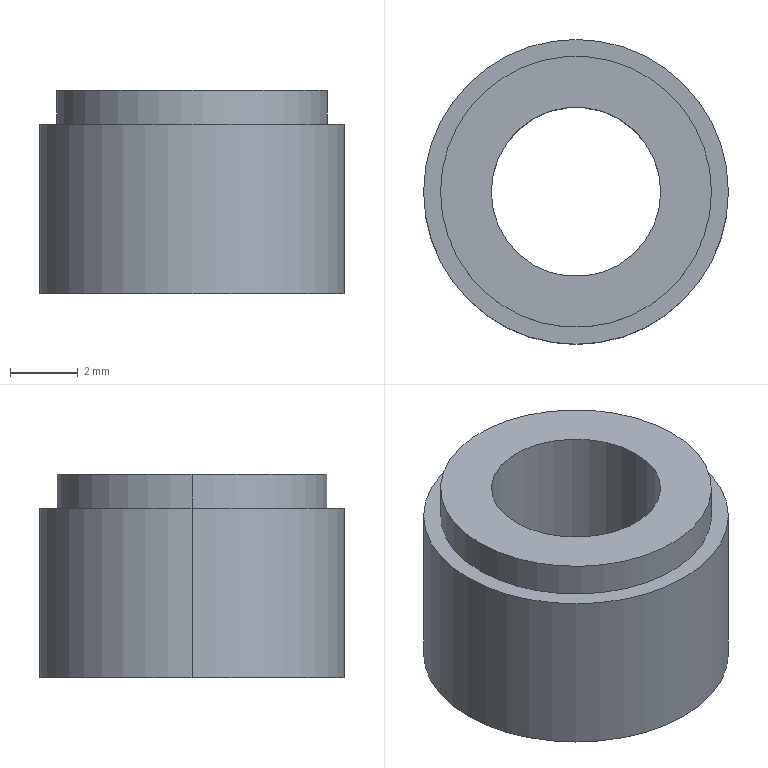Part | SolidWorks | features Extrusion 1, ICE 1 | 1 solid | 9 faces | box 9 x 9 x 6 mm | volume 250.542 mm3 | cylinder 6 | plane 3 | commonest cylinder face diameters 5 x2 8 x2 9 x2
STEP:
#1=CARTESIAN_POINT('',(4.,0.,6.));
#2=VERTEX_POINT('',#1);
#3=CARTESIAN_POINT('',(-4.,0.,6.));
#4=VERTEX_POINT('',#3);
#5=CARTESIAN_POINT('',(0.,0.,6.));
#6=DIRECTION('',(0.,0.,1.));
#7=DIRECTION('',(1.,0.,0.));
#8=AXIS2_PLACEMENT_3D('',#5,#6,#7);
#9=CIRCLE('',#8,4.);
#10=EDGE_CURVE('',#2,#4,#9,.T.);
#11=ORIENTED_EDGE('',*,*,#10,.F.);
#12=CARTESIAN_POINT('',(4.,0.,5.));
#13=VERTEX_POINT('',#12);
#14=CARTESIAN_POINT('',(4.,0.,6.));
#15=DIRECTION('',(0.,0.,-1.));
#16=VECTOR('',#15,1000.);
#17=LINE('',#14,#16);
#18=EDGE_CURVE('',#2,#13,#17,.T.);
#19=ORIENTED_EDGE('',*,*,#18,.T.);
#20=CARTESIAN_POINT('',(-4.,0.,5.));
#21=VERTEX_POINT('',#20);
#22=CARTESIAN_POINT('',(0.,0.,5.));
#23=DIRECTION('',(0.,0.,1.));
#24=DIRECTION('',(1.,0.,0.));
#25=AXIS2_PLACEMENT_3D('',#22,#23,#24);
#26=CIRCLE('',#25,4.);
#27=EDGE_CURVE('',#13,#21,#26,.T.);
#28=ORIENTED_EDGE('',*,*,#27,.T.);
#29=CARTESIAN_POINT('',(-4.,0.,6.));
#30=DIRECTION('',(0.,0.,-1.));
#31=VECTOR('',#30,1000.);
#32=LINE('',#29,#31);
#33=EDGE_CURVE('',#4,#21,#32,.T.);
#34=ORIENTED_EDGE('',*,*,#33,.F.);
#35=EDGE_LOOP('',(#11,#19,#28,#34));
#36=FACE_OUTER_BOUND('',#35,.T.);
#37=CARTESIAN_POINT('',(0.,0.,6.));
#38=DIRECTION('',(0.,0.,-1.));
#39=DIRECTION('',(-1.,0.,0.));
#40=AXIS2_PLACEMENT_3D('',#37,#38,#39);
#41=CYLINDRICAL_SURFACE('',#40,4.);
#42=ADVANCED_FACE('',(#36),#41,.T.);
#43=CARTESIAN_POINT('',(-2.5,0.,6.));
#44=VERTEX_POINT('',#43);
#45=CARTESIAN_POINT('',(2.5,0.,6.));
#46=VERTEX_POINT('',#45);
#47=CARTESIAN_POINT('',(0.,0.,6.));
#48=DIRECTION('',(0.,0.,1.));
#49=DIRECTION('',(1.,0.,0.));
#50=AXIS2_PLACEMENT_3D('',#47,#48,#49);
#51=CIRCLE('',#50,2.5);
#52=EDGE_CURVE('',#44,#46,#51,.T.);
#53=ORIENTED_EDGE('',*,*,#52,.T.);
#54=CARTESIAN_POINT('',(2.5,0.,0.));
#55=VERTEX_POINT('',#54);
#56=CARTESIAN_POINT('',(2.5,0.,5.));
#57=DIRECTION('',(0.,0.,-1.));
#58=VECTOR('',#57,1000.);
#59=LINE('',#56,#58);
#60=EDGE_CURVE('',#46,#55,#59,.T.);
#61=ORIENTED_EDGE('',*,*,#60,.T.);
#62=CARTESIAN_POINT('',(-2.5,0.,0.));
#63=VERTEX_POINT('',#62);
#64=CARTESIAN_POINT('',(0.,0.,0.));
#65=DIRECTION('',(0.,0.,1.));
#66=DIRECTION('',(1.,0.,0.));
#67=AXIS2_PLACEMENT_3D('',#64,#65,#66);
#68=CIRCLE('',#67,2.5);
#69=EDGE_CURVE('',#63,#55,#68,.T.);
#70=ORIENTED_EDGE('',*,*,#69,.F.);
#71=CARTESIAN_POINT('',(-2.5,0.,5.));
#72=DIRECTION('',(0.,0.,-1.));
#73=VECTOR('',#72,1000.);
#74=LINE('',#71,#73);
#75=EDGE_CURVE('',#44,#63,#74,.T.);
#76=ORIENTED_EDGE('',*,*,#75,.F.);
#77=EDGE_LOOP('',(#53,#61,#70,#76));
#78=FACE_OUTER_BOUND('',#77,.T.);
#79=CARTESIAN_POINT('',(0.,0.,5.));
#80=DIRECTION('',(0.,0.,-1.));
#81=DIRECTION('',(-1.,0.,0.));
#82=AXIS2_PLACEMENT_3D('',#79,#80,#81);
#83=CYLINDRICAL_SURFACE('',#82,2.5);
#84=ADVANCED_FACE('',(#78),#83,.F.);
#85=CARTESIAN_POINT('',(4.5,0.,5.));
#86=VERTEX_POINT('',#85);
#87=CARTESIAN_POINT('',(-4.5,0.,5.));
#88=VERTEX_POINT('',#87);
#89=CARTESIAN_POINT('',(0.,0.,5.));
#90=DIRECTION('',(0.,0.,1.));
#91=DIRECTION('',(1.,0.,0.));
#92=AXIS2_PLACEMENT_3D('',#89,#90,#91);
#93=CIRCLE('',#92,4.5);
#94=EDGE_CURVE('',#86,#88,#93,.T.);
#95=ORIENTED_EDGE('',*,*,#94,.F.);
#96=CARTESIAN_POINT('',(4.5,0.,0.));
#97=VERTEX_POINT('',#96);
#98=CARTESIAN_POINT('',(4.5,0.,5.));
#99=DIRECTION('',(0.,0.,-1.));
#100=VECTOR('',#99,1000.);
#101=LINE('',#98,#100);
#102=EDGE_CURVE('',#86,#97,#101,.T.);
#103=ORIENTED_EDGE('',*,*,#102,.T.);
#104=CARTESIAN_POINT('',(-4.5,0.,0.));
#105=VERTEX_POINT('',#104);
#106=CARTESIAN_POINT('',(0.,0.,0.));
#107=DIRECTION('',(0.,0.,1.));
#108=DIRECTION('',(1.,0.,0.));
#109=AXIS2_PLACEMENT_3D('',#106,#107,#108);
#110=CIRCLE('',#109,4.5);
#111=EDGE_CURVE('',#97,#105,#110,.T.);
#112=ORIENTED_EDGE('',*,*,#111,.T.);
#113=CARTESIAN_POINT('',(-4.5,0.,5.));
#114=DIRECTION('',(0.,0.,-1.));
#115=VECTOR('',#114,1000.);
#116=LINE('',#113,#115);
#117=EDGE_CURVE('',#88,#105,#116,.T.);
#118=ORIENTED_EDGE('',*,*,#117,.F.);
#119=EDGE_LOOP('',(#95,#103,#112,#118));
#120=FACE_OUTER_BOUND('',#119,.T.);
#121=CARTESIAN_POINT('',(0.,0.,5.));
#122=DIRECTION('',(0.,0.,-1.));
#123=DIRECTION('',(-1.,0.,0.));
#124=AXIS2_PLACEMENT_3D('',#121,#122,#123);
#125=CYLINDRICAL_SURFACE('',#124,4.5);
#126=ADVANCED_FACE('',(#120),#125,.T.);
#127=CARTESIAN_POINT('',(0.,0.,5.));
#128=DIRECTION('',(0.,0.,1.));
#129=DIRECTION('',(1.,0.,0.));
#130=AXIS2_PLACEMENT_3D('',#127,#128,#129);
#131=CIRCLE('',#130,4.5);
#132=EDGE_CURVE('',#88,#86,#131,.T.);
#133=ORIENTED_EDGE('',*,*,#132,.T.);
#134=ORIENTED_EDGE('',*,*,#94,.T.);
#135=EDGE_LOOP('',(#133,#134));
#136=FACE_OUTER_BOUND('',#135,.T.);
#137=CARTESIAN_POINT('',(0.,0.,5.));
#138=DIRECTION('',(0.,0.,1.));
#139=DIRECTION('',(1.,0.,0.));
#140=AXIS2_PLACEMENT_3D('',#137,#138,#139);
#141=CIRCLE('',#140,4.);
#142=EDGE_CURVE('',#21,#13,#141,.T.);
#143=ORIENTED_EDGE('',*,*,#142,.F.);
#144=ORIENTED_EDGE('',*,*,#27,.F.);
#145=EDGE_LOOP('',(#143,#144));
#146=FACE_BOUND('',#145,.T.);
#147=CARTESIAN_POINT('',(0.,0.,5.));
#148=DIRECTION('',(0.,0.,1.));
#149=DIRECTION('',(1.,0.,0.));
#150=AXIS2_PLACEMENT_3D('',#147,#148,#149);
#151=PLANE('',#150);
#152=ADVANCED_FACE('',(#136,#146),#151,.T.);
#153=CARTESIAN_POINT('',(0.,0.,0.));
#154=DIRECTION('',(0.,0.,1.));
#155=DIRECTION('',(1.,0.,0.));
#156=AXIS2_PLACEMENT_3D('',#153,#154,#155);
#157=CIRCLE('',#156,4.5);
#158=EDGE_CURVE('',#105,#97,#157,.T.);
#159=ORIENTED_EDGE('',*,*,#158,.F.);
#160=ORIENTED_EDGE('',*,*,#111,.F.);
#161=EDGE_LOOP('',(#159,#160));
#162=FACE_OUTER_BOUND('',#161,.T.);
#163=ORIENTED_EDGE('',*,*,#69,.T.);
#164=CARTESIAN_POINT('',(0.,0.,0.));
#165=DIRECTION('',(0.,0.,1.));
#166=DIRECTION('',(1.,0.,0.));
#167=AXIS2_PLACEMENT_3D('',#164,#165,#166);
#168=CIRCLE('',#167,2.5);
#169=EDGE_CURVE('',#55,#63,#168,.T.);
#170=ORIENTED_EDGE('',*,*,#169,.T.);
#171=EDGE_LOOP('',(#163,#170));
#172=FACE_BOUND('',#171,.T.);
#173=CARTESIAN_POINT('',(0.,0.,0.));
#174=DIRECTION('',(0.,0.,1.));
#175=DIRECTION('',(1.,0.,0.));
#176=AXIS2_PLACEMENT_3D('',#173,#174,#175);
#177=PLANE('',#176);
#178=ADVANCED_FACE('',(#162,#172),#177,.F.);
#179=ORIENTED_EDGE('',*,*,#102,.F.);
#180=ORIENTED_EDGE('',*,*,#132,.F.);
#181=ORIENTED_EDGE('',*,*,#117,.T.);
#182=ORIENTED_EDGE('',*,*,#158,.T.);
#183=EDGE_LOOP('',(#179,#180,#181,#182));
#184=FACE_OUTER_BOUND('',#183,.T.);
#185=CARTESIAN_POINT('',(0.,0.,5.));
#186=DIRECTION('',(0.,0.,-1.));
#187=DIRECTION('',(-1.,0.,0.));
#188=AXIS2_PLACEMENT_3D('',#185,#186,#187);
#189=CYLINDRICAL_SURFACE('',#188,4.5);
#190=ADVANCED_FACE('',(#184),#189,.T.);
#191=ORIENTED_EDGE('',*,*,#60,.F.);
#192=CARTESIAN_POINT('',(0.,0.,6.));
#193=DIRECTION('',(0.,0.,1.));
#194=DIRECTION('',(1.,0.,0.));
#195=AXIS2_PLACEMENT_3D('',#192,#193,#194);
#196=CIRCLE('',#195,2.5);
#197=EDGE_CURVE('',#46,#44,#196,.T.);
#198=ORIENTED_EDGE('',*,*,#197,.T.);
#199=ORIENTED_EDGE('',*,*,#75,.T.);
#200=ORIENTED_EDGE('',*,*,#169,.F.);
#201=EDGE_LOOP('',(#191,#198,#199,#200));
#202=FACE_OUTER_BOUND('',#201,.T.);
#203=CARTESIAN_POINT('',(0.,0.,5.));
#204=DIRECTION('',(0.,0.,-1.));
#205=DIRECTION('',(-1.,0.,0.));
#206=AXIS2_PLACEMENT_3D('',#203,#204,#205);
#207=CYLINDRICAL_SURFACE('',#206,2.5);
#208=ADVANCED_FACE('',(#202),#207,.F.);
#209=CARTESIAN_POINT('',(0.,0.,6.));
#210=DIRECTION('',(0.,0.,1.));
#211=DIRECTION('',(1.,0.,0.));
#212=AXIS2_PLACEMENT_3D('',#209,#210,#211);
#213=CIRCLE('',#212,4.);
#214=EDGE_CURVE('',#4,#2,#213,.T.);
#215=ORIENTED_EDGE('',*,*,#214,.T.);
#216=ORIENTED_EDGE('',*,*,#10,.T.);
#217=EDGE_LOOP('',(#215,#216));
#218=FACE_OUTER_BOUND('',#217,.T.);
#219=ORIENTED_EDGE('',*,*,#52,.F.);
#220=ORIENTED_EDGE('',*,*,#197,.F.);
#221=EDGE_LOOP('',(#219,#220));
#222=FACE_BOUND('',#221,.T.);
#223=CARTESIAN_POINT('',(0.,0.,6.));
#224=DIRECTION('',(0.,0.,1.));
#225=DIRECTION('',(1.,0.,0.));
#226=AXIS2_PLACEMENT_3D('',#223,#224,#225);
#227=PLANE('',#226);
#228=ADVANCED_FACE('',(#218,#222),#227,.T.);
#229=ORIENTED_EDGE('',*,*,#18,.F.);
#230=ORIENTED_EDGE('',*,*,#214,.F.);
#231=ORIENTED_EDGE('',*,*,#33,.T.);
#232=ORIENTED_EDGE('',*,*,#142,.T.);
#233=EDGE_LOOP('',(#229,#230,#231,#232));
#234=FACE_OUTER_BOUND('',#233,.T.);
#235=CARTESIAN_POINT('',(0.,0.,6.));
#236=DIRECTION('',(0.,0.,-1.));
#237=DIRECTION('',(-1.,0.,0.));
#238=AXIS2_PLACEMENT_3D('',#235,#236,#237);
#239=CYLINDRICAL_SURFACE('',#238,4.);
#240=ADVANCED_FACE('',(#234),#239,.T.);
#241=CLOSED_SHELL('',(#42,#84,#126,#152,#178,#190,#208,#228,#240));
#242=MANIFOLD_SOLID_BREP('',#241);
#243=CARTESIAN_POINT('',(0.,0.,0.));
#244=DIRECTION('',(0.,0.,1.));
#245=DIRECTION('',(1.,0.,0.));
#246=AXIS2_PLACEMENT_3D('',#243,#244,#245);
#247=(LENGTH_UNIT()NAMED_UNIT(*)SI_UNIT(.MILLI.,.METRE.));
#248=UNCERTAINTY_MEASURE_WITH_UNIT(LENGTH_MEASURE(0.00001),#247,'','');
#249=(NAMED_UNIT(*)PLANE_ANGLE_UNIT()SI_UNIT($,.RADIAN.));
#250=(NAMED_UNIT(*)SI_UNIT($,.STERADIAN.)SOLID_ANGLE_UNIT());
#251=(GEOMETRIC_REPRESENTATION_CONTEXT(3)GLOBAL_UNCERTAINTY_ASSIGNED_CONTEXT((#248))GLOBAL_UNIT_ASSIGNED_CONTEXT((#247,#249,#250))REPRESENTATION_CONTEXT('',''));
#252=ADVANCED_BREP_SHAPE_REPRESENTATION('',(#242,#246),#251);